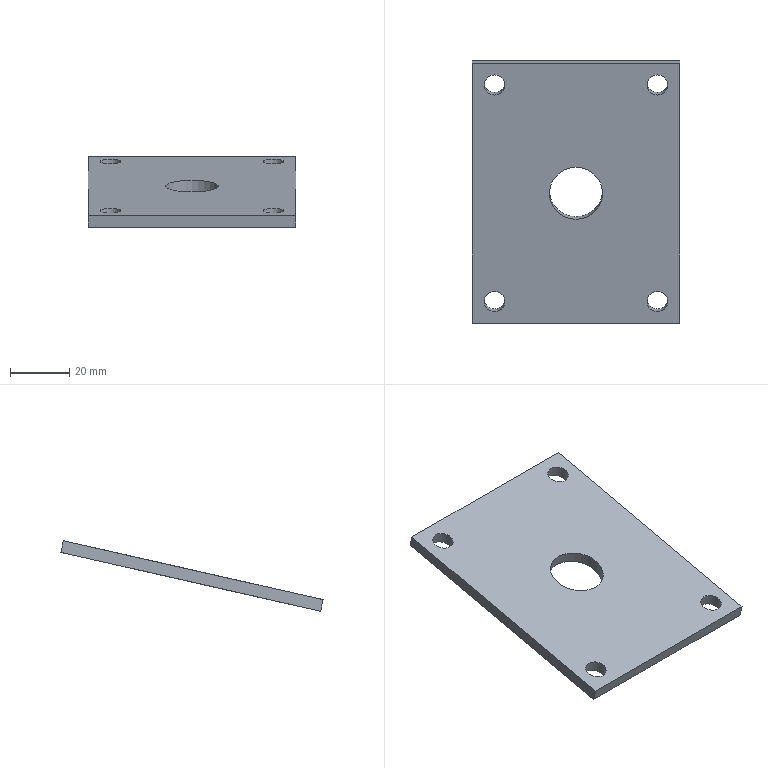Part | NX | features DATUM_CSYS 39, SIMPLE HOLE 38, SKETCH 38, EXTRACT_DATUM_AXIS 32, EXTRACT_FACE 26, HOLE PACKAGE 25, EXTRUDE 22, EXTRACT_DATUM_PLANE 14, Instance Feature 10, DRAFT 8, EXTRACT_STRING 8, BLEND 5, FSET 4, Mirror Feature 4, REPLACE_FACE 4, OFFSET_REGION 3, CPROJ 2, Pattern Feature 2, DATUM_PLANE 1, TRIM BODY 1 | 1 solid | 11 faces | box 70 x 88.654 x 23.816 mm | volume 23566 mm3 | plane 6 | cylinder 5 | commonest cylinder face diameters 7 x4 18 x1
STEP:
#1=CARTESIAN_POINT('',(0.,46.506,94.637));
#2=VERTEX_POINT('',#1);
#3=CARTESIAN_POINT('',(0.,37.729,92.645));
#4=DIRECTION('',(0.,0.2213,-0.9752));
#5=DIRECTION('',(0.,0.9752,0.2213));
#6=AXIS2_PLACEMENT_3D('',#3,#4,#5);
#7=CIRCLE('',#6,9.);
#8=EDGE_CURVE('',#2,#2,#7,.F.);
#9=ORIENTED_EDGE('',*,*,#8,.T.);
#10=EDGE_LOOP('',(#9));
#11=FACE_BOUND('',#10,.T.);
#12=CARTESIAN_POINT('',(-35.,81.613,102.603));
#13=VERTEX_POINT('',#12);
#14=CARTESIAN_POINT('',(-35.,-6.156,82.688));
#15=VERTEX_POINT('',#14);
#16=CARTESIAN_POINT('',(-35.,81.613,102.603));
#17=DIRECTION('',(0.,-0.9752,-0.2213));
#18=VECTOR('',#17,1000.);
#19=LINE('',#16,#18);
#20=EDGE_CURVE('',#13,#15,#19,.T.);
#21=ORIENTED_EDGE('',*,*,#20,.F.);
#22=CARTESIAN_POINT('',(35.,81.613,102.603));
#23=VERTEX_POINT('',#22);
#24=CARTESIAN_POINT('',(35.,81.613,102.603));
#25=DIRECTION('',(-1.,0.,0.));
#26=VECTOR('',#25,1000.);
#27=LINE('',#24,#26);
#28=EDGE_CURVE('',#23,#13,#27,.T.);
#29=ORIENTED_EDGE('',*,*,#28,.F.);
#30=CARTESIAN_POINT('',(35.,-6.156,82.688));
#31=VERTEX_POINT('',#30);
#32=CARTESIAN_POINT('',(35.,-6.156,82.688));
#33=DIRECTION('',(0.,0.9752,0.2213));
#34=VECTOR('',#33,1000.);
#35=LINE('',#32,#34);
#36=EDGE_CURVE('',#31,#23,#35,.T.);
#37=ORIENTED_EDGE('',*,*,#36,.F.);
#38=CARTESIAN_POINT('',(-35.,-6.156,82.688));
#39=DIRECTION('',(1.,0.,0.));
#40=VECTOR('',#39,1000.);
#41=LINE('',#38,#40);
#42=EDGE_CURVE('',#15,#31,#41,.T.);
#43=ORIENTED_EDGE('',*,*,#42,.F.);
#44=EDGE_LOOP('',(#21,#29,#37,#43));
#45=FACE_BOUND('',#44,.T.);
#46=CARTESIAN_POINT('',(-27.5,4.572,85.122));
#47=VERTEX_POINT('',#46);
#48=CARTESIAN_POINT('',(-27.5,1.158,84.347));
#49=DIRECTION('',(0.,0.2213,-0.9752));
#50=DIRECTION('',(0.,0.9752,0.2213));
#51=AXIS2_PLACEMENT_3D('',#48,#49,#50);
#52=CIRCLE('',#51,3.5);
#53=EDGE_CURVE('',#47,#47,#52,.F.);
#54=ORIENTED_EDGE('',*,*,#53,.T.);
#55=EDGE_LOOP('',(#54));
#56=FACE_BOUND('',#55,.T.);
#57=CARTESIAN_POINT('',(27.5,4.572,85.122));
#58=VERTEX_POINT('',#57);
#59=CARTESIAN_POINT('',(27.5,1.158,84.347));
#60=DIRECTION('',(0.,0.2213,-0.9752));
#61=DIRECTION('',(0.,0.9752,0.2213));
#62=AXIS2_PLACEMENT_3D('',#59,#60,#61);
#63=CIRCLE('',#62,3.5);
#64=EDGE_CURVE('',#58,#58,#63,.T.);
#65=ORIENTED_EDGE('',*,*,#64,.F.);
#66=EDGE_LOOP('',(#65));
#67=FACE_BOUND('',#66,.T.);
#68=CARTESIAN_POINT('',(-27.5,77.712,101.717));
#69=VERTEX_POINT('',#68);
#70=CARTESIAN_POINT('',(-27.5,74.299,100.943));
#71=DIRECTION('',(0.,0.2213,-0.9752));
#72=DIRECTION('',(0.,0.9752,0.2213));
#73=AXIS2_PLACEMENT_3D('',#70,#71,#72);
#74=CIRCLE('',#73,3.5);
#75=EDGE_CURVE('',#69,#69,#74,.T.);
#76=ORIENTED_EDGE('',*,*,#75,.F.);
#77=EDGE_LOOP('',(#76));
#78=FACE_BOUND('',#77,.T.);
#79=CARTESIAN_POINT('',(27.5,77.712,101.717));
#80=VERTEX_POINT('',#79);
#81=CARTESIAN_POINT('',(27.5,74.299,100.943));
#82=DIRECTION('',(0.,0.2213,-0.9752));
#83=DIRECTION('',(0.,0.9752,0.2213));
#84=AXIS2_PLACEMENT_3D('',#81,#82,#83);
#85=CIRCLE('',#84,3.5);
#86=EDGE_CURVE('',#80,#80,#85,.F.);
#87=ORIENTED_EDGE('',*,*,#86,.T.);
#88=EDGE_LOOP('',(#87));
#89=FACE_BOUND('',#88,.T.);
#90=CARTESIAN_POINT('',(0.,37.729,92.645));
#91=DIRECTION('',(0.,0.2213,-0.9752));
#92=DIRECTION('',(0.,0.9752,0.2213));
#93=AXIS2_PLACEMENT_3D('',#90,#91,#92);
#94=PLANE('',#93);
#95=ADVANCED_FACE('',(#11,#45,#56,#67,#78,#89),#94,.T.);
#96=CARTESIAN_POINT('',(27.5,76.827,105.618));
#97=VERTEX_POINT('',#96);
#98=CARTESIAN_POINT('',(27.5,73.414,104.844));
#99=DIRECTION('',(0.,0.2213,-0.9752));
#100=DIRECTION('',(0.,0.9752,0.2213));
#101=AXIS2_PLACEMENT_3D('',#98,#99,#100);
#102=CIRCLE('',#101,3.5);
#103=EDGE_CURVE('',#97,#97,#102,.T.);
#104=ORIENTED_EDGE('',*,*,#103,.F.);
#105=EDGE_LOOP('',(#104));
#106=FACE_BOUND('',#105,.T.);
#107=ORIENTED_EDGE('',*,*,#86,.F.);
#108=EDGE_LOOP('',(#107));
#109=FACE_BOUND('',#108,.T.);
#110=CARTESIAN_POINT('',(27.5,73.414,104.844));
#111=DIRECTION('',(0.,0.2213,-0.9752));
#112=DIRECTION('',(0.,0.9752,0.2213));
#113=AXIS2_PLACEMENT_3D('',#110,#111,#112);
#114=CYLINDRICAL_SURFACE('',#113,3.5);
#115=ADVANCED_FACE('',(#106,#109),#114,.F.);
#116=CARTESIAN_POINT('',(-27.5,76.827,105.618));
#117=VERTEX_POINT('',#116);
#118=CARTESIAN_POINT('',(-27.5,73.414,104.844));
#119=DIRECTION('',(0.,-0.2213,0.9752));
#120=DIRECTION('',(0.,0.9752,0.2213));
#121=AXIS2_PLACEMENT_3D('',#118,#119,#120);
#122=CIRCLE('',#121,3.5);
#123=EDGE_CURVE('',#117,#117,#122,.T.);
#124=ORIENTED_EDGE('',*,*,#123,.T.);
#125=EDGE_LOOP('',(#124));
#126=FACE_BOUND('',#125,.T.);
#127=ORIENTED_EDGE('',*,*,#75,.T.);
#128=EDGE_LOOP('',(#127));
#129=FACE_BOUND('',#128,.T.);
#130=CARTESIAN_POINT('',(-27.5,73.414,104.844));
#131=DIRECTION('',(0.,0.2213,-0.9752));
#132=DIRECTION('',(0.,0.9752,0.2213));
#133=AXIS2_PLACEMENT_3D('',#130,#131,#132);
#134=CYLINDRICAL_SURFACE('',#133,3.5);
#135=ADVANCED_FACE('',(#126,#129),#134,.F.);
#136=CARTESIAN_POINT('',(-27.5,-3.14,87.474));
#137=VERTEX_POINT('',#136);
#138=CARTESIAN_POINT('',(-27.5,0.2732,88.248));
#139=DIRECTION('',(0.,0.2213,-0.9752));
#140=DIRECTION('',(0.,-0.9752,-0.2213));
#141=AXIS2_PLACEMENT_3D('',#138,#139,#140);
#142=CIRCLE('',#141,3.5);
#143=EDGE_CURVE('',#137,#137,#142,.T.);
#144=ORIENTED_EDGE('',*,*,#143,.F.);
#145=EDGE_LOOP('',(#144));
#146=FACE_BOUND('',#145,.T.);
#147=ORIENTED_EDGE('',*,*,#53,.F.);
#148=EDGE_LOOP('',(#147));
#149=FACE_BOUND('',#148,.T.);
#150=CARTESIAN_POINT('',(-27.5,0.2732,88.248));
#151=DIRECTION('',(0.,0.2213,-0.9752));
#152=DIRECTION('',(0.,0.9752,0.2213));
#153=AXIS2_PLACEMENT_3D('',#150,#151,#152);
#154=CYLINDRICAL_SURFACE('',#153,3.5);
#155=ADVANCED_FACE('',(#146,#149),#154,.F.);
#156=CARTESIAN_POINT('',(27.5,-3.14,87.474));
#157=VERTEX_POINT('',#156);
#158=CARTESIAN_POINT('',(27.5,0.2732,88.248));
#159=DIRECTION('',(0.,-0.2213,0.9752));
#160=DIRECTION('',(0.,-0.9752,-0.2213));
#161=AXIS2_PLACEMENT_3D('',#158,#159,#160);
#162=CIRCLE('',#161,3.5);
#163=EDGE_CURVE('',#157,#157,#162,.T.);
#164=ORIENTED_EDGE('',*,*,#163,.T.);
#165=EDGE_LOOP('',(#164));
#166=FACE_BOUND('',#165,.T.);
#167=ORIENTED_EDGE('',*,*,#64,.T.);
#168=EDGE_LOOP('',(#167));
#169=FACE_BOUND('',#168,.T.);
#170=CARTESIAN_POINT('',(27.5,0.2732,88.248));
#171=DIRECTION('',(0.,0.2213,-0.9752));
#172=DIRECTION('',(0.,0.9752,0.2213));
#173=AXIS2_PLACEMENT_3D('',#170,#171,#172);
#174=CYLINDRICAL_SURFACE('',#173,3.5);
#175=ADVANCED_FACE('',(#166,#169),#174,.F.);
#176=ORIENTED_EDGE('',*,*,#20,.T.);
#177=CARTESIAN_POINT('',(-35.,-7.041,86.588));
#178=VERTEX_POINT('',#177);
#179=CARTESIAN_POINT('',(-35.,-7.041,86.588));
#180=DIRECTION('',(0.,0.2213,-0.9752));
#181=VECTOR('',#180,1000.);
#182=LINE('',#179,#181);
#183=EDGE_CURVE('',#178,#15,#182,.T.);
#184=ORIENTED_EDGE('',*,*,#183,.F.);
#185=CARTESIAN_POINT('',(-35.,80.728,106.503));
#186=VERTEX_POINT('',#185);
#187=CARTESIAN_POINT('',(-35.,80.728,106.503));
#188=DIRECTION('',(0.,-0.9752,-0.2213));
#189=VECTOR('',#188,1000.);
#190=LINE('',#187,#189);
#191=EDGE_CURVE('',#186,#178,#190,.T.);
#192=ORIENTED_EDGE('',*,*,#191,.F.);
#193=CARTESIAN_POINT('',(-35.,80.728,106.503));
#194=DIRECTION('',(0.,0.2213,-0.9752));
#195=VECTOR('',#194,1000.);
#196=LINE('',#193,#195);
#197=EDGE_CURVE('',#186,#13,#196,.T.);
#198=ORIENTED_EDGE('',*,*,#197,.T.);
#199=EDGE_LOOP('',(#176,#184,#192,#198));
#200=FACE_BOUND('',#199,.T.);
#201=CARTESIAN_POINT('',(-35.,80.728,106.503));
#202=DIRECTION('',(1.,0.,0.));
#203=DIRECTION('',(0.,0.,-1.));
#204=AXIS2_PLACEMENT_3D('',#201,#202,#203);
#205=PLANE('',#204);
#206=ADVANCED_FACE('',(#200),#205,.F.);
#207=ORIENTED_EDGE('',*,*,#42,.T.);
#208=CARTESIAN_POINT('',(35.,-7.041,86.588));
#209=VERTEX_POINT('',#208);
#210=CARTESIAN_POINT('',(35.,-7.041,86.588));
#211=DIRECTION('',(0.,0.2213,-0.9752));
#212=VECTOR('',#211,1000.);
#213=LINE('',#210,#212);
#214=EDGE_CURVE('',#209,#31,#213,.T.);
#215=ORIENTED_EDGE('',*,*,#214,.F.);
#216=CARTESIAN_POINT('',(-35.,-7.041,86.588));
#217=DIRECTION('',(1.,0.,0.));
#218=VECTOR('',#217,1000.);
#219=LINE('',#216,#218);
#220=EDGE_CURVE('',#178,#209,#219,.T.);
#221=ORIENTED_EDGE('',*,*,#220,.F.);
#222=ORIENTED_EDGE('',*,*,#183,.T.);
#223=EDGE_LOOP('',(#207,#215,#221,#222));
#224=FACE_BOUND('',#223,.T.);
#225=CARTESIAN_POINT('',(-35.,-7.041,86.588));
#226=DIRECTION('',(0.,0.9752,0.2213));
#227=DIRECTION('',(0.,-0.2213,0.9752));
#228=AXIS2_PLACEMENT_3D('',#225,#226,#227);
#229=PLANE('',#228);
#230=ADVANCED_FACE('',(#224),#229,.F.);
#231=ORIENTED_EDGE('',*,*,#36,.T.);
#232=CARTESIAN_POINT('',(35.,80.728,106.503));
#233=VERTEX_POINT('',#232);
#234=CARTESIAN_POINT('',(35.,80.728,106.503));
#235=DIRECTION('',(0.,0.2213,-0.9752));
#236=VECTOR('',#235,1000.);
#237=LINE('',#234,#236);
#238=EDGE_CURVE('',#233,#23,#237,.T.);
#239=ORIENTED_EDGE('',*,*,#238,.F.);
#240=CARTESIAN_POINT('',(35.,-7.041,86.588));
#241=DIRECTION('',(0.,0.9752,0.2213));
#242=VECTOR('',#241,1000.);
#243=LINE('',#240,#242);
#244=EDGE_CURVE('',#209,#233,#243,.T.);
#245=ORIENTED_EDGE('',*,*,#244,.F.);
#246=ORIENTED_EDGE('',*,*,#214,.T.);
#247=EDGE_LOOP('',(#231,#239,#245,#246));
#248=FACE_BOUND('',#247,.T.);
#249=CARTESIAN_POINT('',(35.,-7.041,86.588));
#250=DIRECTION('',(-1.,0.,0.));
#251=DIRECTION('',(0.,0.,1.));
#252=AXIS2_PLACEMENT_3D('',#249,#250,#251);
#253=PLANE('',#252);
#254=ADVANCED_FACE('',(#248),#253,.F.);
#255=ORIENTED_EDGE('',*,*,#28,.T.);
#256=ORIENTED_EDGE('',*,*,#197,.F.);
#257=CARTESIAN_POINT('',(35.,80.728,106.503));
#258=DIRECTION('',(-1.,0.,0.));
#259=VECTOR('',#258,1000.);
#260=LINE('',#257,#259);
#261=EDGE_CURVE('',#233,#186,#260,.T.);
#262=ORIENTED_EDGE('',*,*,#261,.F.);
#263=ORIENTED_EDGE('',*,*,#238,.T.);
#264=EDGE_LOOP('',(#255,#256,#262,#263));
#265=FACE_BOUND('',#264,.T.);
#266=CARTESIAN_POINT('',(35.,80.728,106.503));
#267=DIRECTION('',(0.,-0.9752,-0.2213));
#268=DIRECTION('',(0.,0.2213,-0.9752));
#269=AXIS2_PLACEMENT_3D('',#266,#267,#268);
#270=PLANE('',#269);
#271=ADVANCED_FACE('',(#265),#270,.F.);
#272=CARTESIAN_POINT('',(0.,45.621,98.537));
#273=VERTEX_POINT('',#272);
#274=CARTESIAN_POINT('',(0.,36.844,96.546));
#275=DIRECTION('',(0.,0.2213,-0.9752));
#276=DIRECTION('',(0.,0.9752,0.2213));
#277=AXIS2_PLACEMENT_3D('',#274,#275,#276);
#278=CIRCLE('',#277,9.);
#279=EDGE_CURVE('',#273,#273,#278,.F.);
#280=ORIENTED_EDGE('',*,*,#279,.F.);
#281=EDGE_LOOP('',(#280));
#282=FACE_BOUND('',#281,.T.);
#283=ORIENTED_EDGE('',*,*,#191,.T.);
#284=ORIENTED_EDGE('',*,*,#220,.T.);
#285=ORIENTED_EDGE('',*,*,#244,.T.);
#286=ORIENTED_EDGE('',*,*,#261,.T.);
#287=EDGE_LOOP('',(#283,#284,#285,#286));
#288=FACE_BOUND('',#287,.T.);
#289=ORIENTED_EDGE('',*,*,#103,.T.);
#290=EDGE_LOOP('',(#289));
#291=FACE_BOUND('',#290,.T.);
#292=ORIENTED_EDGE('',*,*,#163,.F.);
#293=EDGE_LOOP('',(#292));
#294=FACE_BOUND('',#293,.T.);
#295=ORIENTED_EDGE('',*,*,#123,.F.);
#296=EDGE_LOOP('',(#295));
#297=FACE_BOUND('',#296,.T.);
#298=ORIENTED_EDGE('',*,*,#143,.T.);
#299=EDGE_LOOP('',(#298));
#300=FACE_BOUND('',#299,.T.);
#301=CARTESIAN_POINT('',(27.5,73.414,104.844));
#302=DIRECTION('',(0.,0.2213,-0.9752));
#303=DIRECTION('',(0.,0.9752,0.2213));
#304=AXIS2_PLACEMENT_3D('',#301,#302,#303);
#305=PLANE('',#304);
#306=ADVANCED_FACE('',(#282,#288,#291,#294,#297,#300),#305,.F.);
#307=ORIENTED_EDGE('',*,*,#8,.F.);
#308=EDGE_LOOP('',(#307));
#309=FACE_BOUND('',#308,.T.);
#310=ORIENTED_EDGE('',*,*,#279,.T.);
#311=EDGE_LOOP('',(#310));
#312=FACE_BOUND('',#311,.T.);
#313=CARTESIAN_POINT('',(0.,5.865,233.075));
#314=DIRECTION('',(0.,0.2213,-0.9752));
#315=DIRECTION('',(0.,0.9752,0.2213));
#316=AXIS2_PLACEMENT_3D('',#313,#314,#315);
#317=CYLINDRICAL_SURFACE('',#316,9.);
#318=ADVANCED_FACE('',(#309,#312),#317,.F.);
#319=CLOSED_SHELL('',(#95,#115,#135,#155,#175,#206,#230,#254,#271,#306,#318));
#320=MANIFOLD_SOLID_BREP('',#319);
#321=(LENGTH_UNIT()NAMED_UNIT(*)SI_UNIT(.MILLI.,.METRE.));
#322=UNCERTAINTY_MEASURE_WITH_UNIT(LENGTH_MEASURE(0.00001),#321,'','');
#323=(NAMED_UNIT(*)PLANE_ANGLE_UNIT()SI_UNIT($,.RADIAN.));
#324=(NAMED_UNIT(*)SI_UNIT($,.STERADIAN.)SOLID_ANGLE_UNIT());
#325=(GEOMETRIC_REPRESENTATION_CONTEXT(3)GLOBAL_UNCERTAINTY_ASSIGNED_CONTEXT((#322))GLOBAL_UNIT_ASSIGNED_CONTEXT((#321,#323,#324))REPRESENTATION_CONTEXT('',''));
#326=ADVANCED_BREP_SHAPE_REPRESENTATION('',(#320),#325);